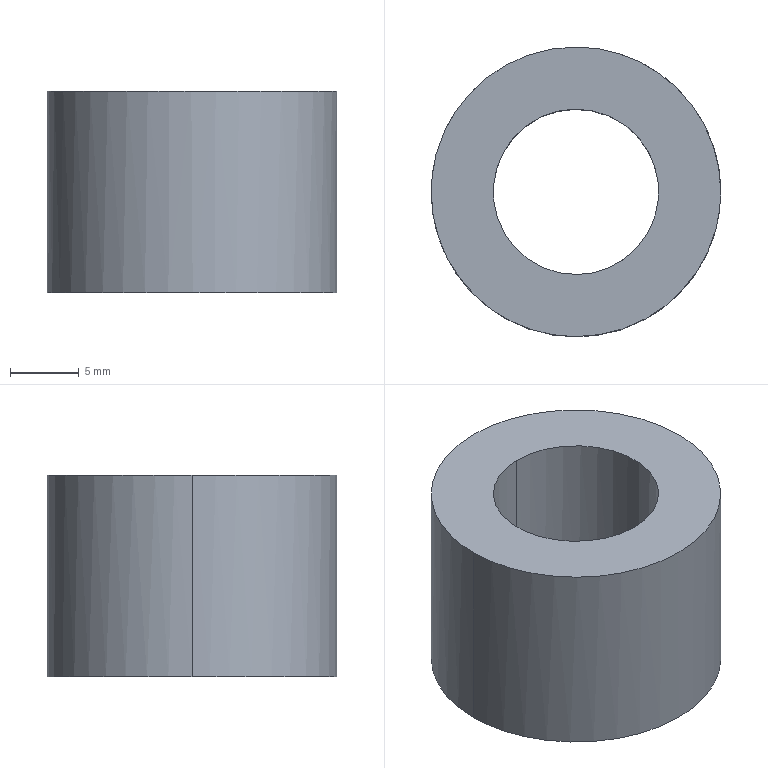Part | SolidWorks | features BaseBody 1 | 1 solid | 6 faces | box 21.004 x 21 x 14.649 mm | volume 3417 mm3 | cylinder 4 | plane 2 | commonest cylinder face diameters 12 x2 21 x2
STEP:
#1=CARTESIAN_POINT('',(341.64,203.402,34.922));
#2=VERTEX_POINT('',#1);
#3=CARTESIAN_POINT('',(341.893,191.405,34.922));
#4=VERTEX_POINT('',#3);
#5=CARTESIAN_POINT('',(341.64,203.402,34.922));
#6=CARTESIAN_POINT('',(353.638,203.655,34.922));
#7=CARTESIAN_POINT('',(353.89,191.657,34.922));
#8=CARTESIAN_POINT('',(341.893,191.405,34.922));
#9=(BOUNDED_CURVE()B_SPLINE_CURVE(3,(#5,#6,#7,#8),.UNSPECIFIED.,.F.,.T.)B_SPLINE_CURVE_WITH_KNOTS((4,4),(4.695,7.837),.UNSPECIFIED.)CURVE()GEOMETRIC_REPRESENTATION_ITEM()RATIONAL_B_SPLINE_CURVE((1.,0.3333,0.3333,1.))REPRESENTATION_ITEM(''));
#10=EDGE_CURVE('',#2,#4,#9,.T.);
#11=ORIENTED_EDGE('',*,*,#10,.F.);
#12=CARTESIAN_POINT('',(341.643,203.402,20.275));
#13=VERTEX_POINT('',#12);
#14=CARTESIAN_POINT('',(341.643,203.402,20.275));
#15=DIRECTION('',(0.0001435,0.000000521,-1.));
#16=VECTOR('',#15,1000.);
#17=LINE('',#14,#16);
#18=EDGE_CURVE('',#2,#13,#17,.T.);
#19=ORIENTED_EDGE('',*,*,#18,.T.);
#20=CARTESIAN_POINT('',(341.895,191.405,20.275));
#21=VERTEX_POINT('',#20);
#22=CARTESIAN_POINT('',(341.769,197.404,20.275));
#23=DIRECTION('',(-0.0001435,-0.000000521,1.));
#24=DIRECTION('',(0.02104,-0.9998,0.000002497));
#25=AXIS2_PLACEMENT_3D('',#22,#23,#24);
#26=CIRCLE('',#25,6.);
#27=EDGE_CURVE('',#21,#13,#26,.T.);
#28=ORIENTED_EDGE('',*,*,#27,.F.);
#29=CARTESIAN_POINT('',(341.895,191.405,20.275));
#30=DIRECTION('',(0.0001435,0.000000521,-1.));
#31=VECTOR('',#30,1000.);
#32=LINE('',#29,#31);
#33=EDGE_CURVE('',#4,#21,#32,.T.);
#34=ORIENTED_EDGE('',*,*,#33,.F.);
#35=EDGE_LOOP('',(#11,#19,#28,#34));
#36=FACE_OUTER_BOUND('',#35,.T.);
#37=CARTESIAN_POINT('',(341.769,197.404,20.275));
#38=DIRECTION('',(0.0001435,0.000000521,-1.));
#39=DIRECTION('',(0.02104,-0.9998,0.000002497));
#40=AXIS2_PLACEMENT_3D('',#37,#38,#39);
#41=CYLINDRICAL_SURFACE('',#40,6.);
#42=ADVANCED_FACE('',(#36),#41,.F.);
#43=CARTESIAN_POINT('',(331.264,197.404,34.922));
#44=VERTEX_POINT('',#43);
#45=CARTESIAN_POINT('',(352.265,197.404,34.922));
#46=VERTEX_POINT('',#45);
#47=CARTESIAN_POINT('',(331.264,197.404,34.922));
#48=CARTESIAN_POINT('',(331.264,176.403,34.922));
#49=CARTESIAN_POINT('',(352.265,176.403,34.922));
#50=CARTESIAN_POINT('',(352.265,197.404,34.922));
#51=(BOUNDED_CURVE()B_SPLINE_CURVE(3,(#47,#48,#49,#50),.UNSPECIFIED.,.F.,.F.)B_SPLINE_CURVE_WITH_KNOTS((4,4),(3.138,6.28),.UNSPECIFIED.)CURVE()GEOMETRIC_REPRESENTATION_ITEM()RATIONAL_B_SPLINE_CURVE((1.,0.3333,0.3333,1.))REPRESENTATION_ITEM(''));
#52=EDGE_CURVE('',#44,#46,#51,.T.);
#53=ORIENTED_EDGE('',*,*,#52,.F.);
#54=CARTESIAN_POINT('',(331.268,197.404,20.273));
#55=VERTEX_POINT('',#54);
#56=CARTESIAN_POINT('',(331.266,197.404,27.273));
#57=DIRECTION('',(0.0002869,0.000001042,-1.));
#58=VECTOR('',#57,1000.);
#59=LINE('',#56,#58);
#60=EDGE_CURVE('',#44,#55,#59,.T.);
#61=ORIENTED_EDGE('',*,*,#60,.T.);
#62=CARTESIAN_POINT('',(352.269,197.404,20.276));
#63=VERTEX_POINT('',#62);
#64=CARTESIAN_POINT('',(352.269,197.404,20.276));
#65=CARTESIAN_POINT('',(352.269,176.403,20.276));
#66=CARTESIAN_POINT('',(331.268,176.403,20.273));
#67=CARTESIAN_POINT('',(331.268,197.404,20.273));
#68=(BOUNDED_CURVE()B_SPLINE_CURVE(3,(#64,#65,#66,#67),.UNSPECIFIED.,.F.,.T.)B_SPLINE_CURVE_WITH_KNOTS((4,4),(0.003633,3.145),.UNSPECIFIED.)CURVE()GEOMETRIC_REPRESENTATION_ITEM()RATIONAL_B_SPLINE_CURVE((1.,0.3333,0.3333,1.))REPRESENTATION_ITEM(''));
#69=EDGE_CURVE('',#63,#55,#68,.T.);
#70=ORIENTED_EDGE('',*,*,#69,.F.);
#71=CARTESIAN_POINT('',(352.267,197.404,27.279));
#72=DIRECTION('',(0.0002869,0.000001042,-1.));
#73=VECTOR('',#72,1000.);
#74=LINE('',#71,#73);
#75=EDGE_CURVE('',#46,#63,#74,.T.);
#76=ORIENTED_EDGE('',*,*,#75,.F.);
#77=EDGE_LOOP('',(#53,#61,#70,#76));
#78=FACE_OUTER_BOUND('',#77,.T.);
#79=CARTESIAN_POINT('',(341.767,197.404,27.276));
#80=DIRECTION('',(0.0002869,0.000001042,-1.));
#81=DIRECTION('',(1.,0.,0.0002869));
#82=AXIS2_PLACEMENT_3D('',#79,#80,#81);
#83=CYLINDRICAL_SURFACE('',#82,10.5);
#84=ADVANCED_FACE('',(#78),#83,.T.);
#85=ORIENTED_EDGE('',*,*,#60,.F.);
#86=CARTESIAN_POINT('',(352.264,197.442,34.922));
#87=VERTEX_POINT('',#86);
#88=CARTESIAN_POINT('',(352.264,197.442,34.922));
#89=CARTESIAN_POINT('',(352.188,218.366,34.922));
#90=CARTESIAN_POINT('',(331.264,218.328,34.922));
#91=CARTESIAN_POINT('',(331.264,197.404,34.922));
#92=(BOUNDED_CURVE()B_SPLINE_CURVE(3,(#88,#89,#90,#91),.UNSPECIFIED.,.F.,.F.)B_SPLINE_CURVE_WITH_KNOTS((4,4),(0.,3.138),.UNSPECIFIED.)CURVE()GEOMETRIC_REPRESENTATION_ITEM()RATIONAL_B_SPLINE_CURVE((1.,0.3345,0.3345,1.))REPRESENTATION_ITEM(''));
#93=EDGE_CURVE('',#87,#44,#92,.T.);
#94=ORIENTED_EDGE('',*,*,#93,.F.);
#95=CARTESIAN_POINT('',(341.764,197.404,34.919));
#96=DIRECTION('',(-0.0002869,-0.000001042,1.));
#97=DIRECTION('',(1.,0.,0.0002869));
#98=AXIS2_PLACEMENT_3D('',#95,#96,#97);
#99=CIRCLE('',#98,10.5);
#100=EDGE_CURVE('',#46,#87,#99,.T.);
#101=ORIENTED_EDGE('',*,*,#100,.F.);
#102=ORIENTED_EDGE('',*,*,#75,.T.);
#103=CARTESIAN_POINT('',(352.269,197.442,20.276));
#104=VERTEX_POINT('',#103);
#105=CARTESIAN_POINT('',(341.769,197.404,20.273));
#106=DIRECTION('',(0.0002869,0.000001042,-1.));
#107=DIRECTION('',(1.,0.003633,0.000287));
#108=AXIS2_PLACEMENT_3D('',#105,#106,#107);
#109=CIRCLE('',#108,10.5);
#110=EDGE_CURVE('',#104,#63,#109,.T.);
#111=ORIENTED_EDGE('',*,*,#110,.F.);
#112=CARTESIAN_POINT('',(331.268,197.404,20.273));
#113=CARTESIAN_POINT('',(331.268,218.328,20.273));
#114=CARTESIAN_POINT('',(352.193,218.366,20.276));
#115=CARTESIAN_POINT('',(352.269,197.442,20.276));
#116=(BOUNDED_CURVE()B_SPLINE_CURVE(3,(#112,#113,#114,#115),.UNSPECIFIED.,.F.,.T.)B_SPLINE_CURVE_WITH_KNOTS((4,4),(3.145,6.283),.UNSPECIFIED.)CURVE()GEOMETRIC_REPRESENTATION_ITEM()RATIONAL_B_SPLINE_CURVE((1.,0.3345,0.3345,1.))REPRESENTATION_ITEM(''));
#117=EDGE_CURVE('',#55,#104,#116,.T.);
#118=ORIENTED_EDGE('',*,*,#117,.F.);
#119=EDGE_LOOP('',(#85,#94,#101,#102,#111,#118));
#120=FACE_OUTER_BOUND('',#119,.T.);
#121=CARTESIAN_POINT('',(341.767,197.404,27.276));
#122=DIRECTION('',(0.0002869,0.000001042,-1.));
#123=DIRECTION('',(1.,0.,0.0002869));
#124=AXIS2_PLACEMENT_3D('',#121,#122,#123);
#125=CYLINDRICAL_SURFACE('',#124,10.5);
#126=ADVANCED_FACE('',(#120),#125,.T.);
#127=CARTESIAN_POINT('',(341.893,191.405,34.922));
#128=CARTESIAN_POINT('',(329.896,191.152,34.922));
#129=CARTESIAN_POINT('',(329.643,203.15,34.922));
#130=CARTESIAN_POINT('',(341.64,203.402,34.922));
#131=(BOUNDED_CURVE()B_SPLINE_CURVE(3,(#127,#128,#129,#130),.UNSPECIFIED.,.F.,.T.)B_SPLINE_CURVE_WITH_KNOTS((4,4),(1.553,4.695),.UNSPECIFIED.)CURVE()GEOMETRIC_REPRESENTATION_ITEM()RATIONAL_B_SPLINE_CURVE((1.,0.3333,0.3333,1.))REPRESENTATION_ITEM(''));
#132=EDGE_CURVE('',#4,#2,#131,.T.);
#133=ORIENTED_EDGE('',*,*,#132,.T.);
#134=ORIENTED_EDGE('',*,*,#10,.T.);
#135=EDGE_LOOP('',(#133,#134));
#136=FACE_BOUND('',#135,.T.);
#137=ORIENTED_EDGE('',*,*,#100,.T.);
#138=ORIENTED_EDGE('',*,*,#93,.T.);
#139=ORIENTED_EDGE('',*,*,#52,.T.);
#140=EDGE_LOOP('',(#137,#138,#139));
#141=FACE_OUTER_BOUND('',#140,.T.);
#142=CARTESIAN_POINT('',(330.292,234.89,34.922));
#143=DIRECTION('',(0.,0.,1.));
#144=DIRECTION('',(1.,0.,0.));
#145=AXIS2_PLACEMENT_3D('',#142,#143,#144);
#146=PLANE('',#145);
#147=ADVANCED_FACE('',(#136,#141),#146,.T.);
#148=ORIENTED_EDGE('',*,*,#18,.F.);
#149=ORIENTED_EDGE('',*,*,#132,.F.);
#150=ORIENTED_EDGE('',*,*,#33,.T.);
#151=CARTESIAN_POINT('',(341.769,197.404,20.275));
#152=DIRECTION('',(-0.0001435,-0.000000521,1.));
#153=DIRECTION('',(0.02104,-0.9998,0.000002497));
#154=AXIS2_PLACEMENT_3D('',#151,#152,#153);
#155=CIRCLE('',#154,6.);
#156=EDGE_CURVE('',#13,#21,#155,.T.);
#157=ORIENTED_EDGE('',*,*,#156,.F.);
#158=EDGE_LOOP('',(#148,#149,#150,#157));
#159=FACE_OUTER_BOUND('',#158,.T.);
#160=CARTESIAN_POINT('',(341.769,197.404,20.275));
#161=DIRECTION('',(0.0001435,0.000000521,-1.));
#162=DIRECTION('',(0.02104,-0.9998,0.000002497));
#163=AXIS2_PLACEMENT_3D('',#160,#161,#162);
#164=CYLINDRICAL_SURFACE('',#163,6.);
#165=ADVANCED_FACE('',(#159),#164,.F.);
#166=ORIENTED_EDGE('',*,*,#27,.T.);
#167=ORIENTED_EDGE('',*,*,#156,.T.);
#168=EDGE_LOOP('',(#166,#167));
#169=FACE_BOUND('',#168,.T.);
#170=ORIENTED_EDGE('',*,*,#69,.T.);
#171=ORIENTED_EDGE('',*,*,#117,.T.);
#172=ORIENTED_EDGE('',*,*,#110,.T.);
#173=EDGE_LOOP('',(#170,#171,#172));
#174=FACE_OUTER_BOUND('',#173,.T.);
#175=CARTESIAN_POINT('',(341.769,197.404,20.275));
#176=DIRECTION('',(-0.0001435,-0.000000521,1.));
#177=DIRECTION('',(-0.003633,1.,0.));
#178=AXIS2_PLACEMENT_3D('',#175,#176,#177);
#179=PLANE('',#178);
#180=ADVANCED_FACE('',(#169,#174),#179,.F.);
#181=CLOSED_SHELL('',(#42,#84,#126,#147,#165,#180));
#182=MANIFOLD_SOLID_BREP('',#181);
#183=CARTESIAN_POINT('',(0.,0.,0.));
#184=DIRECTION('',(0.,0.,1.));
#185=DIRECTION('',(1.,0.,0.));
#186=AXIS2_PLACEMENT_3D('',#183,#184,#185);
#187=(LENGTH_UNIT()NAMED_UNIT(*)SI_UNIT(.MILLI.,.METRE.));
#188=UNCERTAINTY_MEASURE_WITH_UNIT(LENGTH_MEASURE(0.00001),#187,'','');
#189=(NAMED_UNIT(*)PLANE_ANGLE_UNIT()SI_UNIT($,.RADIAN.));
#190=(NAMED_UNIT(*)SI_UNIT($,.STERADIAN.)SOLID_ANGLE_UNIT());
#191=(GEOMETRIC_REPRESENTATION_CONTEXT(3)GLOBAL_UNCERTAINTY_ASSIGNED_CONTEXT((#188))GLOBAL_UNIT_ASSIGNED_CONTEXT((#187,#189,#190))REPRESENTATION_CONTEXT('',''));
#192=ADVANCED_BREP_SHAPE_REPRESENTATION('',(#182,#186),#191);